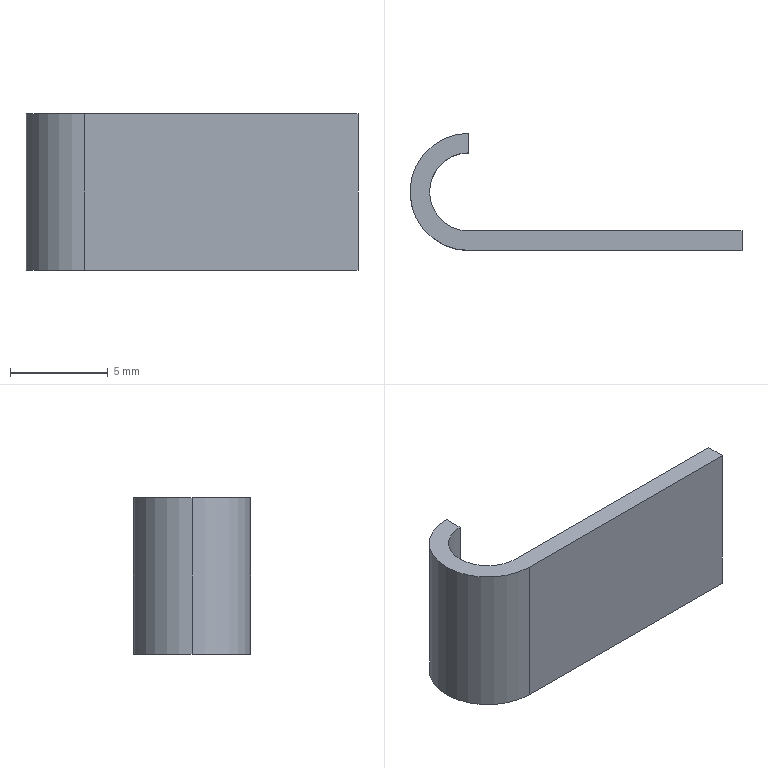Part | SolidWorks | features Extrusion 1 | 1 solid | 10 faces | box 17 x 6 x 8 mm | volume 174.832 mm3 | plane 6 | cylinder 4 | commonest cylinder face diameters 4 x2 6 x2
STEP:
#1=CARTESIAN_POINT('',(-18.538,-38.507,8.));
#2=VERTEX_POINT('',#1);
#3=CARTESIAN_POINT('',(-15.538,-41.507,8.));
#4=VERTEX_POINT('',#3);
#5=CARTESIAN_POINT('',(-15.538,-38.507,8.));
#6=DIRECTION('',(0.,0.,1.));
#7=DIRECTION('',(1.,0.,0.));
#8=AXIS2_PLACEMENT_3D('',#5,#6,#7);
#9=CIRCLE('',#8,3.);
#10=EDGE_CURVE('',#2,#4,#9,.T.);
#11=ORIENTED_EDGE('',*,*,#10,.F.);
#12=CARTESIAN_POINT('',(-18.538,-38.507,0.));
#13=VERTEX_POINT('',#12);
#14=CARTESIAN_POINT('',(-18.538,-38.507,8.));
#15=DIRECTION('',(0.,0.,-1.));
#16=VECTOR('',#15,1000.);
#17=LINE('',#14,#16);
#18=EDGE_CURVE('',#2,#13,#17,.T.);
#19=ORIENTED_EDGE('',*,*,#18,.T.);
#20=CARTESIAN_POINT('',(-15.538,-41.507,0.));
#21=VERTEX_POINT('',#20);
#22=CARTESIAN_POINT('',(-15.538,-38.507,0.));
#23=DIRECTION('',(0.,0.,1.));
#24=DIRECTION('',(1.,0.,0.));
#25=AXIS2_PLACEMENT_3D('',#22,#23,#24);
#26=CIRCLE('',#25,3.);
#27=EDGE_CURVE('',#13,#21,#26,.T.);
#28=ORIENTED_EDGE('',*,*,#27,.T.);
#29=CARTESIAN_POINT('',(-15.538,-41.507,8.));
#30=DIRECTION('',(0.,0.,-1.));
#31=VECTOR('',#30,1000.);
#32=LINE('',#29,#31);
#33=EDGE_CURVE('',#4,#21,#32,.T.);
#34=ORIENTED_EDGE('',*,*,#33,.F.);
#35=EDGE_LOOP('',(#11,#19,#28,#34));
#36=FACE_OUTER_BOUND('',#35,.T.);
#37=CARTESIAN_POINT('',(-15.538,-38.507,8.));
#38=DIRECTION('',(0.,0.,-1.));
#39=DIRECTION('',(-1.,0.,0.));
#40=AXIS2_PLACEMENT_3D('',#37,#38,#39);
#41=CYLINDRICAL_SURFACE('',#40,3.);
#42=ADVANCED_FACE('',(#36),#41,.T.);
#43=CARTESIAN_POINT('',(-17.538,-38.507,8.));
#44=VERTEX_POINT('',#43);
#45=CARTESIAN_POINT('',(-15.538,-36.507,8.));
#46=VERTEX_POINT('',#45);
#47=CARTESIAN_POINT('',(-15.538,-38.507,8.));
#48=DIRECTION('',(0.,0.,-1.));
#49=DIRECTION('',(1.,0.,0.));
#50=AXIS2_PLACEMENT_3D('',#47,#48,#49);
#51=CIRCLE('',#50,2.);
#52=EDGE_CURVE('',#44,#46,#51,.T.);
#53=ORIENTED_EDGE('',*,*,#52,.F.);
#54=CARTESIAN_POINT('',(-17.538,-38.507,0.));
#55=VERTEX_POINT('',#54);
#56=CARTESIAN_POINT('',(-17.538,-38.507,8.));
#57=DIRECTION('',(0.,0.,-1.));
#58=VECTOR('',#57,1000.);
#59=LINE('',#56,#58);
#60=EDGE_CURVE('',#44,#55,#59,.T.);
#61=ORIENTED_EDGE('',*,*,#60,.T.);
#62=CARTESIAN_POINT('',(-15.538,-36.507,0.));
#63=VERTEX_POINT('',#62);
#64=CARTESIAN_POINT('',(-15.538,-38.507,0.));
#65=DIRECTION('',(0.,0.,-1.));
#66=DIRECTION('',(1.,0.,0.));
#67=AXIS2_PLACEMENT_3D('',#64,#65,#66);
#68=CIRCLE('',#67,2.);
#69=EDGE_CURVE('',#55,#63,#68,.T.);
#70=ORIENTED_EDGE('',*,*,#69,.T.);
#71=CARTESIAN_POINT('',(-15.538,-36.507,8.));
#72=DIRECTION('',(0.,0.,-1.));
#73=VECTOR('',#72,1000.);
#74=LINE('',#71,#73);
#75=EDGE_CURVE('',#46,#63,#74,.T.);
#76=ORIENTED_EDGE('',*,*,#75,.F.);
#77=EDGE_LOOP('',(#53,#61,#70,#76));
#78=FACE_OUTER_BOUND('',#77,.T.);
#79=CARTESIAN_POINT('',(-15.538,-38.507,8.));
#80=DIRECTION('',(0.,0.,-1.));
#81=DIRECTION('',(-1.,0.,0.));
#82=AXIS2_PLACEMENT_3D('',#79,#80,#81);
#83=CYLINDRICAL_SURFACE('',#82,2.);
#84=ADVANCED_FACE('',(#78),#83,.F.);
#85=CARTESIAN_POINT('',(-1.538,-41.507,0.));
#86=VERTEX_POINT('',#85);
#87=CARTESIAN_POINT('',(-1.538,-40.507,0.));
#88=VERTEX_POINT('',#87);
#89=CARTESIAN_POINT('',(-1.538,-40.507,0.));
#90=DIRECTION('',(0.,1.,0.));
#91=VECTOR('',#90,1000.);
#92=LINE('',#89,#91);
#93=EDGE_CURVE('',#86,#88,#92,.T.);
#94=ORIENTED_EDGE('',*,*,#93,.T.);
#95=CARTESIAN_POINT('',(-1.538,-40.507,8.));
#96=VERTEX_POINT('',#95);
#97=CARTESIAN_POINT('',(-1.538,-40.507,8.));
#98=DIRECTION('',(0.,0.,-1.));
#99=VECTOR('',#98,1000.);
#100=LINE('',#97,#99);
#101=EDGE_CURVE('',#96,#88,#100,.T.);
#102=ORIENTED_EDGE('',*,*,#101,.F.);
#103=CARTESIAN_POINT('',(-1.538,-41.507,8.));
#104=VERTEX_POINT('',#103);
#105=CARTESIAN_POINT('',(-1.538,-40.507,8.));
#106=DIRECTION('',(0.,1.,0.));
#107=VECTOR('',#106,1000.);
#108=LINE('',#105,#107);
#109=EDGE_CURVE('',#104,#96,#108,.T.);
#110=ORIENTED_EDGE('',*,*,#109,.F.);
#111=CARTESIAN_POINT('',(-1.538,-41.507,8.));
#112=DIRECTION('',(0.,0.,-1.));
#113=VECTOR('',#112,1000.);
#114=LINE('',#111,#113);
#115=EDGE_CURVE('',#104,#86,#114,.T.);
#116=ORIENTED_EDGE('',*,*,#115,.T.);
#117=EDGE_LOOP('',(#94,#102,#110,#116));
#118=FACE_OUTER_BOUND('',#117,.T.);
#119=CARTESIAN_POINT('',(-1.538,-40.507,8.));
#120=DIRECTION('',(-1.,0.,0.));
#121=DIRECTION('',(0.,0.,1.));
#122=AXIS2_PLACEMENT_3D('',#119,#120,#121);
#123=PLANE('',#122);
#124=ADVANCED_FACE('',(#118),#123,.F.);
#125=CARTESIAN_POINT('',(-15.538,-40.507,0.));
#126=VERTEX_POINT('',#125);
#127=CARTESIAN_POINT('',(-1.538,-40.507,0.));
#128=DIRECTION('',(-1.,0.,0.));
#129=VECTOR('',#128,1000.);
#130=LINE('',#127,#129);
#131=EDGE_CURVE('',#88,#126,#130,.T.);
#132=ORIENTED_EDGE('',*,*,#131,.T.);
#133=CARTESIAN_POINT('',(-15.538,-40.507,8.));
#134=VERTEX_POINT('',#133);
#135=CARTESIAN_POINT('',(-15.538,-40.507,8.));
#136=DIRECTION('',(0.,0.,-1.));
#137=VECTOR('',#136,1000.);
#138=LINE('',#135,#137);
#139=EDGE_CURVE('',#134,#126,#138,.T.);
#140=ORIENTED_EDGE('',*,*,#139,.F.);
#141=CARTESIAN_POINT('',(-1.538,-40.507,8.));
#142=DIRECTION('',(-1.,0.,0.));
#143=VECTOR('',#142,1000.);
#144=LINE('',#141,#143);
#145=EDGE_CURVE('',#96,#134,#144,.T.);
#146=ORIENTED_EDGE('',*,*,#145,.F.);
#147=ORIENTED_EDGE('',*,*,#101,.T.);
#148=EDGE_LOOP('',(#132,#140,#146,#147));
#149=FACE_OUTER_BOUND('',#148,.T.);
#150=CARTESIAN_POINT('',(-1.538,-40.507,8.));
#151=DIRECTION('',(0.,-1.,0.));
#152=DIRECTION('',(0.,0.,-1.));
#153=AXIS2_PLACEMENT_3D('',#150,#151,#152);
#154=PLANE('',#153);
#155=ADVANCED_FACE('',(#149),#154,.F.);
#156=ORIENTED_EDGE('',*,*,#60,.F.);
#157=CARTESIAN_POINT('',(-15.538,-38.507,8.));
#158=DIRECTION('',(0.,0.,-1.));
#159=DIRECTION('',(1.,0.,0.));
#160=AXIS2_PLACEMENT_3D('',#157,#158,#159);
#161=CIRCLE('',#160,2.);
#162=EDGE_CURVE('',#134,#44,#161,.T.);
#163=ORIENTED_EDGE('',*,*,#162,.F.);
#164=ORIENTED_EDGE('',*,*,#139,.T.);
#165=CARTESIAN_POINT('',(-15.538,-38.507,0.));
#166=DIRECTION('',(0.,0.,-1.));
#167=DIRECTION('',(1.,0.,0.));
#168=AXIS2_PLACEMENT_3D('',#165,#166,#167);
#169=CIRCLE('',#168,2.);
#170=EDGE_CURVE('',#126,#55,#169,.T.);
#171=ORIENTED_EDGE('',*,*,#170,.T.);
#172=EDGE_LOOP('',(#156,#163,#164,#171));
#173=FACE_OUTER_BOUND('',#172,.T.);
#174=CARTESIAN_POINT('',(-15.538,-38.507,8.));
#175=DIRECTION('',(0.,0.,-1.));
#176=DIRECTION('',(-1.,0.,0.));
#177=AXIS2_PLACEMENT_3D('',#174,#175,#176);
#178=CYLINDRICAL_SURFACE('',#177,2.);
#179=ADVANCED_FACE('',(#173),#178,.F.);
#180=CARTESIAN_POINT('',(-15.538,-35.507,0.));
#181=VERTEX_POINT('',#180);
#182=CARTESIAN_POINT('',(-15.538,-35.507,0.));
#183=DIRECTION('',(0.,1.,0.));
#184=VECTOR('',#183,1000.);
#185=LINE('',#182,#184);
#186=EDGE_CURVE('',#63,#181,#185,.T.);
#187=ORIENTED_EDGE('',*,*,#186,.T.);
#188=CARTESIAN_POINT('',(-15.538,-35.507,8.));
#189=VERTEX_POINT('',#188);
#190=CARTESIAN_POINT('',(-15.538,-35.507,8.));
#191=DIRECTION('',(0.,0.,-1.));
#192=VECTOR('',#191,1000.);
#193=LINE('',#190,#192);
#194=EDGE_CURVE('',#189,#181,#193,.T.);
#195=ORIENTED_EDGE('',*,*,#194,.F.);
#196=CARTESIAN_POINT('',(-15.538,-35.507,8.));
#197=DIRECTION('',(0.,1.,0.));
#198=VECTOR('',#197,1000.);
#199=LINE('',#196,#198);
#200=EDGE_CURVE('',#46,#189,#199,.T.);
#201=ORIENTED_EDGE('',*,*,#200,.F.);
#202=ORIENTED_EDGE('',*,*,#75,.T.);
#203=EDGE_LOOP('',(#187,#195,#201,#202));
#204=FACE_OUTER_BOUND('',#203,.T.);
#205=CARTESIAN_POINT('',(-15.538,-35.507,8.));
#206=DIRECTION('',(-1.,0.,0.));
#207=DIRECTION('',(0.,0.,1.));
#208=AXIS2_PLACEMENT_3D('',#205,#206,#207);
#209=PLANE('',#208);
#210=ADVANCED_FACE('',(#204),#209,.F.);
#211=ORIENTED_EDGE('',*,*,#18,.F.);
#212=CARTESIAN_POINT('',(-15.538,-38.507,8.));
#213=DIRECTION('',(0.,0.,1.));
#214=DIRECTION('',(1.,0.,0.));
#215=AXIS2_PLACEMENT_3D('',#212,#213,#214);
#216=CIRCLE('',#215,3.);
#217=EDGE_CURVE('',#189,#2,#216,.T.);
#218=ORIENTED_EDGE('',*,*,#217,.F.);
#219=ORIENTED_EDGE('',*,*,#194,.T.);
#220=CARTESIAN_POINT('',(-15.538,-38.507,0.));
#221=DIRECTION('',(0.,0.,1.));
#222=DIRECTION('',(1.,0.,0.));
#223=AXIS2_PLACEMENT_3D('',#220,#221,#222);
#224=CIRCLE('',#223,3.);
#225=EDGE_CURVE('',#181,#13,#224,.T.);
#226=ORIENTED_EDGE('',*,*,#225,.T.);
#227=EDGE_LOOP('',(#211,#218,#219,#226));
#228=FACE_OUTER_BOUND('',#227,.T.);
#229=CARTESIAN_POINT('',(-15.538,-38.507,8.));
#230=DIRECTION('',(0.,0.,-1.));
#231=DIRECTION('',(-1.,0.,0.));
#232=AXIS2_PLACEMENT_3D('',#229,#230,#231);
#233=CYLINDRICAL_SURFACE('',#232,3.);
#234=ADVANCED_FACE('',(#228),#233,.T.);
#235=CARTESIAN_POINT('',(-1.538,-41.507,0.));
#236=DIRECTION('',(1.,0.,0.));
#237=VECTOR('',#236,1000.);
#238=LINE('',#235,#237);
#239=EDGE_CURVE('',#21,#86,#238,.T.);
#240=ORIENTED_EDGE('',*,*,#239,.T.);
#241=ORIENTED_EDGE('',*,*,#115,.F.);
#242=CARTESIAN_POINT('',(-1.538,-41.507,8.));
#243=DIRECTION('',(1.,0.,0.));
#244=VECTOR('',#243,1000.);
#245=LINE('',#242,#244);
#246=EDGE_CURVE('',#4,#104,#245,.T.);
#247=ORIENTED_EDGE('',*,*,#246,.F.);
#248=ORIENTED_EDGE('',*,*,#33,.T.);
#249=EDGE_LOOP('',(#240,#241,#247,#248));
#250=FACE_OUTER_BOUND('',#249,.T.);
#251=CARTESIAN_POINT('',(-1.538,-41.507,8.));
#252=DIRECTION('',(0.,1.,0.));
#253=DIRECTION('',(0.,0.,1.));
#254=AXIS2_PLACEMENT_3D('',#251,#252,#253);
#255=PLANE('',#254);
#256=ADVANCED_FACE('',(#250),#255,.F.);
#257=ORIENTED_EDGE('',*,*,#109,.T.);
#258=ORIENTED_EDGE('',*,*,#145,.T.);
#259=ORIENTED_EDGE('',*,*,#162,.T.);
#260=ORIENTED_EDGE('',*,*,#52,.T.);
#261=ORIENTED_EDGE('',*,*,#200,.T.);
#262=ORIENTED_EDGE('',*,*,#217,.T.);
#263=ORIENTED_EDGE('',*,*,#10,.T.);
#264=ORIENTED_EDGE('',*,*,#246,.T.);
#265=EDGE_LOOP('',(#257,#258,#259,#260,#261,#262,#263,#264));
#266=FACE_OUTER_BOUND('',#265,.T.);
#267=CARTESIAN_POINT('',(-15.538,-38.507,8.));
#268=DIRECTION('',(0.,0.,1.));
#269=DIRECTION('',(1.,0.,0.));
#270=AXIS2_PLACEMENT_3D('',#267,#268,#269);
#271=PLANE('',#270);
#272=ADVANCED_FACE('',(#266),#271,.T.);
#273=ORIENTED_EDGE('',*,*,#93,.F.);
#274=ORIENTED_EDGE('',*,*,#239,.F.);
#275=ORIENTED_EDGE('',*,*,#27,.F.);
#276=ORIENTED_EDGE('',*,*,#225,.F.);
#277=ORIENTED_EDGE('',*,*,#186,.F.);
#278=ORIENTED_EDGE('',*,*,#69,.F.);
#279=ORIENTED_EDGE('',*,*,#170,.F.);
#280=ORIENTED_EDGE('',*,*,#131,.F.);
#281=EDGE_LOOP('',(#273,#274,#275,#276,#277,#278,#279,#280));
#282=FACE_OUTER_BOUND('',#281,.T.);
#283=CARTESIAN_POINT('',(-15.538,-38.507,0.));
#284=DIRECTION('',(0.,0.,1.));
#285=DIRECTION('',(1.,0.,0.));
#286=AXIS2_PLACEMENT_3D('',#283,#284,#285);
#287=PLANE('',#286);
#288=ADVANCED_FACE('',(#282),#287,.F.);
#289=CLOSED_SHELL('',(#42,#84,#124,#155,#179,#210,#234,#256,#272,#288));
#290=MANIFOLD_SOLID_BREP('',#289);
#291=CARTESIAN_POINT('',(0.,0.,0.));
#292=DIRECTION('',(0.,0.,1.));
#293=DIRECTION('',(1.,0.,0.));
#294=AXIS2_PLACEMENT_3D('',#291,#292,#293);
#295=(LENGTH_UNIT()NAMED_UNIT(*)SI_UNIT(.MILLI.,.METRE.));
#296=UNCERTAINTY_MEASURE_WITH_UNIT(LENGTH_MEASURE(0.00001),#295,'','');
#297=(NAMED_UNIT(*)PLANE_ANGLE_UNIT()SI_UNIT($,.RADIAN.));
#298=(NAMED_UNIT(*)SI_UNIT($,.STERADIAN.)SOLID_ANGLE_UNIT());
#299=(GEOMETRIC_REPRESENTATION_CONTEXT(3)GLOBAL_UNCERTAINTY_ASSIGNED_CONTEXT((#296))GLOBAL_UNIT_ASSIGNED_CONTEXT((#295,#297,#298))REPRESENTATION_CONTEXT('',''));
#300=ADVANCED_BREP_SHAPE_REPRESENTATION('',(#290,#294),#299);